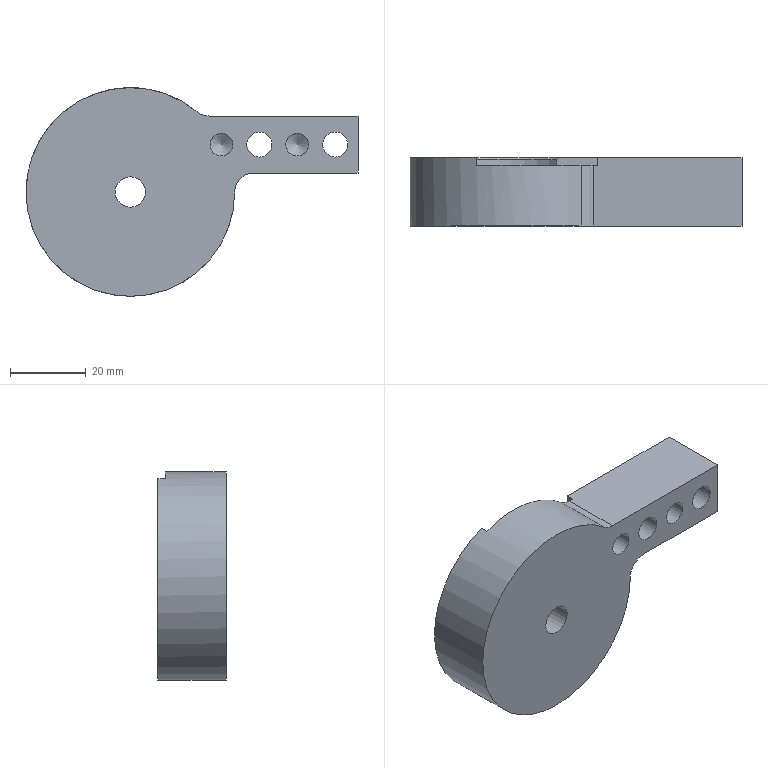Part | NX | features BREP 1 | 1 solid | 26 faces | box 87.5 x 18 x 55 mm | volume 41559 mm3 | plane 12 | cylinder 11 | cone 3 | commonest cylinder face diameters 6 x2 6.6 x2 10 x2 11 x2 8 x1 30 x1
STEP:
#1=CARTESIAN_POINT('',(17.572,7.,21.154));
#2=VERTEX_POINT('',#1);
#3=CARTESIAN_POINT('',(20.767,7.,20.));
#4=VERTEX_POINT('',#3);
#5=CARTESIAN_POINT('',(20.767,7.,25.));
#6=DIRECTION('',(0.,-1.,0.));
#7=DIRECTION('',(0.,0.,1.));
#8=AXIS2_PLACEMENT_3D('',#5,#6,#7);
#9=CIRCLE('',#8,5.);
#10=EDGE_CURVE('',#2,#4,#9,.T.);
#11=ORIENTED_EDGE('',*,*,#10,.F.);
#12=CARTESIAN_POINT('',(17.572,-9.,21.154));
#13=VERTEX_POINT('',#12);
#14=CARTESIAN_POINT('',(17.572,9.,21.154));
#15=DIRECTION('',(0.,1.,0.));
#16=VECTOR('',#15,1000.);
#17=LINE('',#14,#16);
#18=EDGE_CURVE('',#13,#2,#17,.T.);
#19=ORIENTED_EDGE('',*,*,#18,.F.);
#20=CARTESIAN_POINT('',(20.767,-9.,20.));
#21=VERTEX_POINT('',#20);
#22=CARTESIAN_POINT('',(20.767,-9.,25.));
#23=DIRECTION('',(0.,1.,0.));
#24=DIRECTION('',(0.,0.,1.));
#25=AXIS2_PLACEMENT_3D('',#22,#23,#24);
#26=CIRCLE('',#25,5.);
#27=EDGE_CURVE('',#21,#13,#26,.T.);
#28=ORIENTED_EDGE('',*,*,#27,.F.);
#29=CARTESIAN_POINT('',(20.767,-9.,20.));
#30=DIRECTION('',(0.,-1.,0.));
#31=VECTOR('',#30,1000.);
#32=LINE('',#29,#31);
#33=EDGE_CURVE('',#4,#21,#32,.T.);
#34=ORIENTED_EDGE('',*,*,#33,.F.);
#35=EDGE_LOOP('',(#11,#19,#28,#34));
#36=FACE_BOUND('',#35,.T.);
#37=CARTESIAN_POINT('',(20.767,9.,25.));
#38=DIRECTION('',(0.,-1.,0.));
#39=DIRECTION('',(0.,0.,1.));
#40=AXIS2_PLACEMENT_3D('',#37,#38,#39);
#41=CYLINDRICAL_SURFACE('',#40,5.);
#42=ADVANCED_FACE('',(#36),#41,.F.);
#43=CARTESIAN_POINT('',(-10.,7.,25.617));
#44=VERTEX_POINT('',#43);
#45=CARTESIAN_POINT('',(0.,7.,0.));
#46=DIRECTION('',(0.,1.,0.));
#47=DIRECTION('',(0.,0.,1.));
#48=AXIS2_PLACEMENT_3D('',#45,#46,#47);
#49=CIRCLE('',#48,27.5);
#50=EDGE_CURVE('',#44,#2,#49,.T.);
#51=ORIENTED_EDGE('',*,*,#50,.F.);
#52=CARTESIAN_POINT('',(-10.,9.,25.617));
#53=VERTEX_POINT('',#52);
#54=CARTESIAN_POINT('',(-10.,9.,25.617));
#55=DIRECTION('',(0.,1.,0.));
#56=VECTOR('',#55,1000.);
#57=LINE('',#54,#56);
#58=EDGE_CURVE('',#44,#53,#57,.T.);
#59=ORIENTED_EDGE('',*,*,#58,.T.);
#60=CARTESIAN_POINT('',(27.5,9.,0.));
#61=VERTEX_POINT('',#60);
#62=CARTESIAN_POINT('',(0.,9.,0.));
#63=DIRECTION('',(0.,1.,0.));
#64=DIRECTION('',(0.,0.,1.));
#65=AXIS2_PLACEMENT_3D('',#62,#63,#64);
#66=CIRCLE('',#65,27.5);
#67=EDGE_CURVE('',#61,#53,#66,.T.);
#68=ORIENTED_EDGE('',*,*,#67,.F.);
#69=CARTESIAN_POINT('',(27.5,-9.,0.));
#70=VERTEX_POINT('',#69);
#71=CARTESIAN_POINT('',(27.5,9.,0.));
#72=DIRECTION('',(0.,-1.,0.));
#73=VECTOR('',#72,1000.);
#74=LINE('',#71,#73);
#75=EDGE_CURVE('',#61,#70,#74,.T.);
#76=ORIENTED_EDGE('',*,*,#75,.T.);
#77=CARTESIAN_POINT('',(0.,-9.,0.));
#78=DIRECTION('',(0.,1.,0.));
#79=DIRECTION('',(0.,0.,1.));
#80=AXIS2_PLACEMENT_3D('',#77,#78,#79);
#81=CIRCLE('',#80,27.5);
#82=EDGE_CURVE('',#70,#13,#81,.T.);
#83=ORIENTED_EDGE('',*,*,#82,.T.);
#84=ORIENTED_EDGE('',*,*,#18,.T.);
#85=EDGE_LOOP('',(#51,#59,#68,#76,#83,#84));
#86=FACE_BOUND('',#85,.T.);
#87=CARTESIAN_POINT('',(0.,9.,0.));
#88=DIRECTION('',(0.,-1.,0.));
#89=DIRECTION('',(0.,0.,1.));
#90=AXIS2_PLACEMENT_3D('',#87,#88,#89);
#91=CYLINDRICAL_SURFACE('',#90,27.5);
#92=ADVANCED_FACE('',(#86),#91,.T.);
#93=CARTESIAN_POINT('',(-10.,9.,11.843));
#94=VERTEX_POINT('',#93);
#95=CARTESIAN_POINT('',(-10.,9.,10.));
#96=DIRECTION('',(0.,0.,1.));
#97=VECTOR('',#96,1000.);
#98=LINE('',#95,#97);
#99=EDGE_CURVE('',#94,#53,#98,.T.);
#100=ORIENTED_EDGE('',*,*,#99,.F.);
#101=CARTESIAN_POINT('',(11.843,9.,10.));
#102=VERTEX_POINT('',#101);
#103=CARTESIAN_POINT('',(0.,9.,0.));
#104=DIRECTION('',(0.,-1.,0.));
#105=DIRECTION('',(0.,0.,1.));
#106=AXIS2_PLACEMENT_3D('',#103,#104,#105);
#107=CIRCLE('',#106,15.5);
#108=EDGE_CURVE('',#94,#102,#107,.T.);
#109=ORIENTED_EDGE('',*,*,#108,.T.);
#110=CARTESIAN_POINT('',(22.,9.,10.));
#111=VERTEX_POINT('',#110);
#112=CARTESIAN_POINT('',(-10.,9.,10.));
#113=DIRECTION('',(-1.,0.,0.));
#114=VECTOR('',#113,1000.);
#115=LINE('',#112,#114);
#116=EDGE_CURVE('',#111,#102,#115,.T.);
#117=ORIENTED_EDGE('',*,*,#116,.F.);
#118=CARTESIAN_POINT('',(22.,9.,20.));
#119=VERTEX_POINT('',#118);
#120=CARTESIAN_POINT('',(22.,9.,10.));
#121=DIRECTION('',(0.,0.,-1.));
#122=VECTOR('',#121,1000.);
#123=LINE('',#120,#122);
#124=EDGE_CURVE('',#119,#111,#123,.T.);
#125=ORIENTED_EDGE('',*,*,#124,.F.);
#126=CARTESIAN_POINT('',(60.,9.,20.));
#127=VERTEX_POINT('',#126);
#128=CARTESIAN_POINT('',(0.,9.,20.));
#129=DIRECTION('',(1.,0.,0.));
#130=VECTOR('',#129,1000.);
#131=LINE('',#128,#130);
#132=EDGE_CURVE('',#119,#127,#131,.T.);
#133=ORIENTED_EDGE('',*,*,#132,.T.);
#134=CARTESIAN_POINT('',(60.,9.,5.));
#135=VERTEX_POINT('',#134);
#136=CARTESIAN_POINT('',(60.,9.,0.));
#137=DIRECTION('',(0.,0.,1.));
#138=VECTOR('',#137,1000.);
#139=LINE('',#136,#138);
#140=EDGE_CURVE('',#135,#127,#139,.T.);
#141=ORIENTED_EDGE('',*,*,#140,.F.);
#142=CARTESIAN_POINT('',(32.5,9.,5.));
#143=VERTEX_POINT('',#142);
#144=CARTESIAN_POINT('',(0.,9.,5.));
#145=DIRECTION('',(1.,0.,0.));
#146=VECTOR('',#145,1000.);
#147=LINE('',#144,#146);
#148=EDGE_CURVE('',#143,#135,#147,.T.);
#149=ORIENTED_EDGE('',*,*,#148,.F.);
#150=CARTESIAN_POINT('',(32.5,9.,0.));
#151=DIRECTION('',(0.,-1.,0.));
#152=DIRECTION('',(0.,0.,1.));
#153=AXIS2_PLACEMENT_3D('',#150,#151,#152);
#154=CIRCLE('',#153,5.);
#155=EDGE_CURVE('',#143,#61,#154,.T.);
#156=ORIENTED_EDGE('',*,*,#155,.T.);
#157=ORIENTED_EDGE('',*,*,#67,.T.);
#158=EDGE_LOOP('',(#100,#109,#117,#125,#133,#141,#149,#156,#157));
#159=FACE_BOUND('',#158,.T.);
#160=CARTESIAN_POINT('',(34.,9.,18.));
#161=VERTEX_POINT('',#160);
#162=CARTESIAN_POINT('',(34.,9.,12.5));
#163=DIRECTION('',(0.,1.,0.));
#164=DIRECTION('',(0.,0.,1.));
#165=AXIS2_PLACEMENT_3D('',#162,#163,#164);
#166=CIRCLE('',#165,5.5);
#167=EDGE_CURVE('',#161,#161,#166,.T.);
#168=ORIENTED_EDGE('',*,*,#167,.F.);
#169=EDGE_LOOP('',(#168));
#170=FACE_BOUND('',#169,.T.);
#171=CARTESIAN_POINT('',(54.,9.,18.));
#172=VERTEX_POINT('',#171);
#173=CARTESIAN_POINT('',(54.,9.,12.5));
#174=DIRECTION('',(0.,1.,0.));
#175=DIRECTION('',(0.,0.,1.));
#176=AXIS2_PLACEMENT_3D('',#173,#174,#175);
#177=CIRCLE('',#176,5.5);
#178=EDGE_CURVE('',#172,#172,#177,.T.);
#179=ORIENTED_EDGE('',*,*,#178,.F.);
#180=EDGE_LOOP('',(#179));
#181=FACE_BOUND('',#180,.T.);
#182=CARTESIAN_POINT('',(0.,9.,0.));
#183=DIRECTION('',(0.,1.,0.));
#184=DIRECTION('',(0.,0.,-1.));
#185=AXIS2_PLACEMENT_3D('',#182,#183,#184);
#186=PLANE('',#185);
#187=ADVANCED_FACE('',(#159,#170,#181),#186,.T.);
#188=CARTESIAN_POINT('',(44.,-9.,9.5));
#189=VERTEX_POINT('',#188);
#190=CARTESIAN_POINT('',(44.,-9.,12.5));
#191=DIRECTION('',(0.,-1.,0.));
#192=DIRECTION('',(0.,0.,-1.));
#193=AXIS2_PLACEMENT_3D('',#190,#191,#192);
#194=CIRCLE('',#193,3.);
#195=EDGE_CURVE('',#189,#189,#194,.T.);
#196=ORIENTED_EDGE('',*,*,#195,.F.);
#197=EDGE_LOOP('',(#196));
#198=FACE_BOUND('',#197,.T.);
#199=CARTESIAN_POINT('',(24.,-9.,9.5));
#200=VERTEX_POINT('',#199);
#201=CARTESIAN_POINT('',(24.,-9.,12.5));
#202=DIRECTION('',(0.,-1.,0.));
#203=DIRECTION('',(0.,0.,-1.));
#204=AXIS2_PLACEMENT_3D('',#201,#202,#203);
#205=CIRCLE('',#204,3.);
#206=EDGE_CURVE('',#200,#200,#205,.T.);
#207=ORIENTED_EDGE('',*,*,#206,.F.);
#208=EDGE_LOOP('',(#207));
#209=FACE_BOUND('',#208,.T.);
#210=CARTESIAN_POINT('',(34.,-9.,15.8));
#211=VERTEX_POINT('',#210);
#212=CARTESIAN_POINT('',(34.,-9.,12.5));
#213=DIRECTION('',(0.,1.,0.));
#214=DIRECTION('',(0.,0.,1.));
#215=AXIS2_PLACEMENT_3D('',#212,#213,#214);
#216=CIRCLE('',#215,3.3);
#217=EDGE_CURVE('',#211,#211,#216,.T.);
#218=ORIENTED_EDGE('',*,*,#217,.T.);
#219=EDGE_LOOP('',(#218));
#220=FACE_BOUND('',#219,.T.);
#221=CARTESIAN_POINT('',(54.,-9.,15.8));
#222=VERTEX_POINT('',#221);
#223=CARTESIAN_POINT('',(54.,-9.,12.5));
#224=DIRECTION('',(0.,1.,0.));
#225=DIRECTION('',(0.,0.,1.));
#226=AXIS2_PLACEMENT_3D('',#223,#224,#225);
#227=CIRCLE('',#226,3.3);
#228=EDGE_CURVE('',#222,#222,#227,.T.);
#229=ORIENTED_EDGE('',*,*,#228,.T.);
#230=EDGE_LOOP('',(#229));
#231=FACE_BOUND('',#230,.T.);
#232=CARTESIAN_POINT('',(0.,-9.,4.));
#233=VERTEX_POINT('',#232);
#234=CARTESIAN_POINT('',(0.,-9.,0.));
#235=DIRECTION('',(0.,1.,0.));
#236=DIRECTION('',(0.,0.,1.));
#237=AXIS2_PLACEMENT_3D('',#234,#235,#236);
#238=CIRCLE('',#237,4.);
#239=EDGE_CURVE('',#233,#233,#238,.T.);
#240=ORIENTED_EDGE('',*,*,#239,.T.);
#241=EDGE_LOOP('',(#240));
#242=FACE_BOUND('',#241,.T.);
#243=ORIENTED_EDGE('',*,*,#82,.F.);
#244=CARTESIAN_POINT('',(32.5,-9.,5.));
#245=VERTEX_POINT('',#244);
#246=CARTESIAN_POINT('',(32.5,-9.,0.));
#247=DIRECTION('',(0.,1.,0.));
#248=DIRECTION('',(0.,0.,1.));
#249=AXIS2_PLACEMENT_3D('',#246,#247,#248);
#250=CIRCLE('',#249,5.);
#251=EDGE_CURVE('',#70,#245,#250,.T.);
#252=ORIENTED_EDGE('',*,*,#251,.T.);
#253=CARTESIAN_POINT('',(60.,-9.,5.));
#254=VERTEX_POINT('',#253);
#255=CARTESIAN_POINT('',(0.,-9.,5.));
#256=DIRECTION('',(1.,0.,0.));
#257=VECTOR('',#256,1000.);
#258=LINE('',#255,#257);
#259=EDGE_CURVE('',#245,#254,#258,.T.);
#260=ORIENTED_EDGE('',*,*,#259,.T.);
#261=CARTESIAN_POINT('',(60.,-9.,20.));
#262=VERTEX_POINT('',#261);
#263=CARTESIAN_POINT('',(60.,-9.,0.));
#264=DIRECTION('',(0.,0.,1.));
#265=VECTOR('',#264,1000.);
#266=LINE('',#263,#265);
#267=EDGE_CURVE('',#254,#262,#266,.T.);
#268=ORIENTED_EDGE('',*,*,#267,.T.);
#269=CARTESIAN_POINT('',(0.,-9.,20.));
#270=DIRECTION('',(1.,0.,0.));
#271=VECTOR('',#270,1000.);
#272=LINE('',#269,#271);
#273=EDGE_CURVE('',#21,#262,#272,.T.);
#274=ORIENTED_EDGE('',*,*,#273,.F.);
#275=ORIENTED_EDGE('',*,*,#27,.T.);
#276=EDGE_LOOP('',(#243,#252,#260,#268,#274,#275));
#277=FACE_BOUND('',#276,.T.);
#278=CARTESIAN_POINT('',(0.,-9.,0.));
#279=DIRECTION('',(0.,1.,0.));
#280=DIRECTION('',(0.,0.,-1.));
#281=AXIS2_PLACEMENT_3D('',#278,#279,#280);
#282=PLANE('',#281);
#283=ADVANCED_FACE('',(#198,#209,#220,#231,#242,#277),#282,.F.);
#284=CARTESIAN_POINT('',(60.,52.776,5.));
#285=DIRECTION('',(0.,-1.,0.));
#286=VECTOR('',#285,1000.);
#287=LINE('',#284,#286);
#288=EDGE_CURVE('',#135,#254,#287,.T.);
#289=ORIENTED_EDGE('',*,*,#288,.F.);
#290=ORIENTED_EDGE('',*,*,#140,.T.);
#291=CARTESIAN_POINT('',(60.,52.776,20.));
#292=DIRECTION('',(0.,-1.,0.));
#293=VECTOR('',#292,1000.);
#294=LINE('',#291,#293);
#295=EDGE_CURVE('',#127,#262,#294,.T.);
#296=ORIENTED_EDGE('',*,*,#295,.T.);
#297=ORIENTED_EDGE('',*,*,#267,.F.);
#298=EDGE_LOOP('',(#289,#290,#296,#297));
#299=FACE_BOUND('',#298,.T.);
#300=CARTESIAN_POINT('',(60.,52.776,0.));
#301=DIRECTION('',(1.,0.,0.));
#302=DIRECTION('',(0.,0.,1.));
#303=AXIS2_PLACEMENT_3D('',#300,#301,#302);
#304=PLANE('',#303);
#305=ADVANCED_FACE('',(#299),#304,.T.);
#306=ORIENTED_EDGE('',*,*,#132,.F.);
#307=CARTESIAN_POINT('',(22.,7.,20.));
#308=VERTEX_POINT('',#307);
#309=CARTESIAN_POINT('',(22.,52.776,20.));
#310=DIRECTION('',(0.,-1.,0.));
#311=VECTOR('',#310,1000.);
#312=LINE('',#309,#311);
#313=EDGE_CURVE('',#119,#308,#312,.T.);
#314=ORIENTED_EDGE('',*,*,#313,.T.);
#315=CARTESIAN_POINT('',(0.,7.,20.));
#316=DIRECTION('',(1.,0.,0.));
#317=VECTOR('',#316,1000.);
#318=LINE('',#315,#317);
#319=EDGE_CURVE('',#4,#308,#318,.T.);
#320=ORIENTED_EDGE('',*,*,#319,.F.);
#321=ORIENTED_EDGE('',*,*,#33,.T.);
#322=ORIENTED_EDGE('',*,*,#273,.T.);
#323=ORIENTED_EDGE('',*,*,#295,.F.);
#324=EDGE_LOOP('',(#306,#314,#320,#321,#322,#323));
#325=FACE_BOUND('',#324,.T.);
#326=CARTESIAN_POINT('',(0.,52.776,20.));
#327=DIRECTION('',(0.,0.,-1.));
#328=DIRECTION('',(1.,0.,0.));
#329=AXIS2_PLACEMENT_3D('',#326,#327,#328);
#330=PLANE('',#329);
#331=ADVANCED_FACE('',(#325),#330,.F.);
#332=ORIENTED_EDGE('',*,*,#259,.F.);
#333=CARTESIAN_POINT('',(32.5,52.776,5.));
#334=DIRECTION('',(0.,1.,0.));
#335=VECTOR('',#334,1000.);
#336=LINE('',#333,#335);
#337=EDGE_CURVE('',#245,#143,#336,.T.);
#338=ORIENTED_EDGE('',*,*,#337,.T.);
#339=ORIENTED_EDGE('',*,*,#148,.T.);
#340=ORIENTED_EDGE('',*,*,#288,.T.);
#341=EDGE_LOOP('',(#332,#338,#339,#340));
#342=FACE_BOUND('',#341,.T.);
#343=CARTESIAN_POINT('',(0.,52.776,5.));
#344=DIRECTION('',(0.,0.,-1.));
#345=DIRECTION('',(1.,0.,0.));
#346=AXIS2_PLACEMENT_3D('',#343,#344,#345);
#347=PLANE('',#346);
#348=ADVANCED_FACE('',(#342),#347,.T.);
#349=CARTESIAN_POINT('',(11.18,8.5,10.));
#350=VERTEX_POINT('',#349);
#351=CARTESIAN_POINT('',(-10.,8.5,11.18));
#352=VERTEX_POINT('',#351);
#353=CARTESIAN_POINT('',(0.,8.5,0.));
#354=DIRECTION('',(0.,1.,0.));
#355=DIRECTION('',(0.,0.,1.));
#356=AXIS2_PLACEMENT_3D('',#353,#354,#355);
#357=CIRCLE('',#356,15.);
#358=EDGE_CURVE('',#350,#352,#357,.T.);
#359=ORIENTED_EDGE('',*,*,#358,.T.);
#360=CARTESIAN_POINT('',(-10.,7.,11.18));
#361=VERTEX_POINT('',#360);
#362=CARTESIAN_POINT('',(-10.,-1.,11.18));
#363=DIRECTION('',(0.,-1.,0.));
#364=VECTOR('',#363,1000.);
#365=LINE('',#362,#364);
#366=EDGE_CURVE('',#352,#361,#365,.T.);
#367=ORIENTED_EDGE('',*,*,#366,.T.);
#368=CARTESIAN_POINT('',(11.18,7.,10.));
#369=VERTEX_POINT('',#368);
#370=CARTESIAN_POINT('',(0.,7.,0.));
#371=DIRECTION('',(0.,-1.,0.));
#372=DIRECTION('',(0.,0.,1.));
#373=AXIS2_PLACEMENT_3D('',#370,#371,#372);
#374=CIRCLE('',#373,15.);
#375=EDGE_CURVE('',#369,#361,#374,.T.);
#376=ORIENTED_EDGE('',*,*,#375,.F.);
#377=CARTESIAN_POINT('',(11.18,-1.,10.));
#378=DIRECTION('',(0.,1.,0.));
#379=VECTOR('',#378,1000.);
#380=LINE('',#377,#379);
#381=EDGE_CURVE('',#369,#350,#380,.T.);
#382=ORIENTED_EDGE('',*,*,#381,.T.);
#383=EDGE_LOOP('',(#359,#367,#376,#382));
#384=FACE_BOUND('',#383,.T.);
#385=CARTESIAN_POINT('',(0.,-1.,15.));
#386=VERTEX_POINT('',#385);
#387=CARTESIAN_POINT('',(0.,-1.,0.));
#388=DIRECTION('',(0.,1.,0.));
#389=DIRECTION('',(0.,0.,1.));
#390=AXIS2_PLACEMENT_3D('',#387,#388,#389);
#391=CIRCLE('',#390,15.);
#392=EDGE_CURVE('',#386,#386,#391,.T.);
#393=ORIENTED_EDGE('',*,*,#392,.F.);
#394=EDGE_LOOP('',(#393));
#395=FACE_BOUND('',#394,.T.);
#396=CARTESIAN_POINT('',(0.,-1.,0.));
#397=DIRECTION('',(0.,1.,0.));
#398=DIRECTION('',(0.,0.,-1.));
#399=AXIS2_PLACEMENT_3D('',#396,#397,#398);
#400=CYLINDRICAL_SURFACE('',#399,15.);
#401=ADVANCED_FACE('',(#384,#395),#400,.F.);
#402=CARTESIAN_POINT('',(0.,-1.,4.));
#403=VERTEX_POINT('',#402);
#404=CARTESIAN_POINT('',(0.,-1.,0.));
#405=DIRECTION('',(0.,1.,0.));
#406=DIRECTION('',(0.,0.,1.));
#407=AXIS2_PLACEMENT_3D('',#404,#405,#406);
#408=CIRCLE('',#407,4.);
#409=EDGE_CURVE('',#403,#403,#408,.T.);
#410=ORIENTED_EDGE('',*,*,#409,.F.);
#411=EDGE_LOOP('',(#410));
#412=FACE_BOUND('',#411,.T.);
#413=ORIENTED_EDGE('',*,*,#392,.T.);
#414=EDGE_LOOP('',(#413));
#415=FACE_BOUND('',#414,.T.);
#416=CARTESIAN_POINT('',(0.,-1.,0.));
#417=DIRECTION('',(0.,1.,0.));
#418=DIRECTION('',(0.,0.,-1.));
#419=AXIS2_PLACEMENT_3D('',#416,#417,#418);
#420=PLANE('',#419);
#421=ADVANCED_FACE('',(#412,#415),#420,.T.);
#422=ORIENTED_EDGE('',*,*,#239,.F.);
#423=EDGE_LOOP('',(#422));
#424=FACE_BOUND('',#423,.T.);
#425=ORIENTED_EDGE('',*,*,#409,.T.);
#426=EDGE_LOOP('',(#425));
#427=FACE_BOUND('',#426,.T.);
#428=CARTESIAN_POINT('',(0.,-1.,0.));
#429=DIRECTION('',(0.,1.,0.));
#430=DIRECTION('',(0.,0.,-1.));
#431=AXIS2_PLACEMENT_3D('',#428,#429,#430);
#432=CYLINDRICAL_SURFACE('',#431,4.);
#433=ADVANCED_FACE('',(#424,#427),#432,.F.);
#434=ORIENTED_EDGE('',*,*,#228,.F.);
#435=EDGE_LOOP('',(#434));
#436=FACE_BOUND('',#435,.T.);
#437=CARTESIAN_POINT('',(54.,2.6,15.8));
#438=VERTEX_POINT('',#437);
#439=CARTESIAN_POINT('',(54.,2.6,12.5));
#440=DIRECTION('',(0.,1.,0.));
#441=DIRECTION('',(0.,0.,1.));
#442=AXIS2_PLACEMENT_3D('',#439,#440,#441);
#443=CIRCLE('',#442,3.3);
#444=EDGE_CURVE('',#438,#438,#443,.T.);
#445=ORIENTED_EDGE('',*,*,#444,.T.);
#446=EDGE_LOOP('',(#445));
#447=FACE_BOUND('',#446,.T.);
#448=CARTESIAN_POINT('',(54.,9.,12.5));
#449=DIRECTION('',(0.,1.,0.));
#450=DIRECTION('',(0.,0.,-1.));
#451=AXIS2_PLACEMENT_3D('',#448,#449,#450);
#452=CYLINDRICAL_SURFACE('',#451,3.3);
#453=ADVANCED_FACE('',(#436,#447),#452,.F.);
#454=ORIENTED_EDGE('',*,*,#444,.F.);
#455=EDGE_LOOP('',(#454));
#456=FACE_BOUND('',#455,.T.);
#457=CARTESIAN_POINT('',(54.,2.6,18.));
#458=VERTEX_POINT('',#457);
#459=CARTESIAN_POINT('',(54.,2.6,12.5));
#460=DIRECTION('',(0.,1.,0.));
#461=DIRECTION('',(0.,0.,1.));
#462=AXIS2_PLACEMENT_3D('',#459,#460,#461);
#463=CIRCLE('',#462,5.5);
#464=EDGE_CURVE('',#458,#458,#463,.T.);
#465=ORIENTED_EDGE('',*,*,#464,.T.);
#466=EDGE_LOOP('',(#465));
#467=FACE_BOUND('',#466,.T.);
#468=CARTESIAN_POINT('',(57.3,2.6,12.5));
#469=DIRECTION('',(0.,-1.,0.));
#470=DIRECTION('',(0.,0.,1.));
#471=AXIS2_PLACEMENT_3D('',#468,#469,#470);
#472=PLANE('',#471);
#473=ADVANCED_FACE('',(#456,#467),#472,.F.);
#474=ORIENTED_EDGE('',*,*,#464,.F.);
#475=EDGE_LOOP('',(#474));
#476=FACE_BOUND('',#475,.T.);
#477=ORIENTED_EDGE('',*,*,#178,.T.);
#478=EDGE_LOOP('',(#477));
#479=FACE_BOUND('',#478,.T.);
#480=CARTESIAN_POINT('',(54.,9.,12.5));
#481=DIRECTION('',(0.,1.,0.));
#482=DIRECTION('',(0.,0.,-1.));
#483=AXIS2_PLACEMENT_3D('',#480,#481,#482);
#484=CYLINDRICAL_SURFACE('',#483,5.5);
#485=ADVANCED_FACE('',(#476,#479),#484,.F.);
#486=ORIENTED_EDGE('',*,*,#217,.F.);
#487=EDGE_LOOP('',(#486));
#488=FACE_BOUND('',#487,.T.);
#489=CARTESIAN_POINT('',(34.,2.6,15.8));
#490=VERTEX_POINT('',#489);
#491=CARTESIAN_POINT('',(34.,2.6,12.5));
#492=DIRECTION('',(0.,1.,0.));
#493=DIRECTION('',(0.,0.,1.));
#494=AXIS2_PLACEMENT_3D('',#491,#492,#493);
#495=CIRCLE('',#494,3.3);
#496=EDGE_CURVE('',#490,#490,#495,.T.);
#497=ORIENTED_EDGE('',*,*,#496,.T.);
#498=EDGE_LOOP('',(#497));
#499=FACE_BOUND('',#498,.T.);
#500=CARTESIAN_POINT('',(34.,9.,12.5));
#501=DIRECTION('',(0.,1.,0.));
#502=DIRECTION('',(0.,0.,-1.));
#503=AXIS2_PLACEMENT_3D('',#500,#501,#502);
#504=CYLINDRICAL_SURFACE('',#503,3.3);
#505=ADVANCED_FACE('',(#488,#499),#504,.F.);
#506=ORIENTED_EDGE('',*,*,#496,.F.);
#507=EDGE_LOOP('',(#506));
#508=FACE_BOUND('',#507,.T.);
#509=CARTESIAN_POINT('',(34.,2.6,18.));
#510=VERTEX_POINT('',#509);
#511=CARTESIAN_POINT('',(34.,2.6,12.5));
#512=DIRECTION('',(0.,1.,0.));
#513=DIRECTION('',(0.,0.,1.));
#514=AXIS2_PLACEMENT_3D('',#511,#512,#513);
#515=CIRCLE('',#514,5.5);
#516=EDGE_CURVE('',#510,#510,#515,.T.);
#517=ORIENTED_EDGE('',*,*,#516,.T.);
#518=EDGE_LOOP('',(#517));
#519=FACE_BOUND('',#518,.T.);
#520=CARTESIAN_POINT('',(37.3,2.6,12.5));
#521=DIRECTION('',(0.,-1.,0.));
#522=DIRECTION('',(0.,0.,1.));
#523=AXIS2_PLACEMENT_3D('',#520,#521,#522);
#524=PLANE('',#523);
#525=ADVANCED_FACE('',(#508,#519),#524,.F.);
#526=ORIENTED_EDGE('',*,*,#516,.F.);
#527=EDGE_LOOP('',(#526));
#528=FACE_BOUND('',#527,.T.);
#529=ORIENTED_EDGE('',*,*,#167,.T.);
#530=EDGE_LOOP('',(#529));
#531=FACE_BOUND('',#530,.T.);
#532=CARTESIAN_POINT('',(34.,9.,12.5));
#533=DIRECTION('',(0.,1.,0.));
#534=DIRECTION('',(0.,0.,-1.));
#535=AXIS2_PLACEMENT_3D('',#532,#533,#534);
#536=CYLINDRICAL_SURFACE('',#535,5.5);
#537=ADVANCED_FACE('',(#528,#531),#536,.F.);
#538=CARTESIAN_POINT('',(24.,5.203,12.5));
#539=VERTEX_POINT('',#538);
#540=VERTEX_LOOP('',#539);
#541=FACE_BOUND('',#540,.T.);
#542=CARTESIAN_POINT('',(24.,3.4,9.5));
#543=VERTEX_POINT('',#542);
#544=CARTESIAN_POINT('',(24.,3.4,12.5));
#545=DIRECTION('',(0.,-1.,0.));
#546=DIRECTION('',(0.,0.,-1.));
#547=AXIS2_PLACEMENT_3D('',#544,#545,#546);
#548=CIRCLE('',#547,3.);
#549=EDGE_CURVE('',#543,#543,#548,.T.);
#550=ORIENTED_EDGE('',*,*,#549,.T.);
#551=EDGE_LOOP('',(#550));
#552=FACE_BOUND('',#551,.T.);
#553=CARTESIAN_POINT('',(24.,3.4,12.5));
#554=DIRECTION('',(0.,-1.,0.));
#555=DIRECTION('',(0.,0.,1.));
#556=AXIS2_PLACEMENT_3D('',#553,#554,#555);
#557=CONICAL_SURFACE('',#556,3.,1.03);
#558=ADVANCED_FACE('',(#541,#552),#557,.F.);
#559=ORIENTED_EDGE('',*,*,#549,.F.);
#560=EDGE_LOOP('',(#559));
#561=FACE_BOUND('',#560,.T.);
#562=ORIENTED_EDGE('',*,*,#206,.T.);
#563=EDGE_LOOP('',(#562));
#564=FACE_BOUND('',#563,.T.);
#565=CARTESIAN_POINT('',(24.,-9.,12.5));
#566=DIRECTION('',(0.,-1.,0.));
#567=DIRECTION('',(0.,0.,1.));
#568=AXIS2_PLACEMENT_3D('',#565,#566,#567);
#569=CYLINDRICAL_SURFACE('',#568,3.);
#570=ADVANCED_FACE('',(#561,#564),#569,.F.);
#571=CARTESIAN_POINT('',(44.,5.203,12.5));
#572=VERTEX_POINT('',#571);
#573=VERTEX_LOOP('',#572);
#574=FACE_BOUND('',#573,.T.);
#575=CARTESIAN_POINT('',(44.,3.4,9.5));
#576=VERTEX_POINT('',#575);
#577=CARTESIAN_POINT('',(44.,3.4,12.5));
#578=DIRECTION('',(0.,-1.,0.));
#579=DIRECTION('',(0.,0.,-1.));
#580=AXIS2_PLACEMENT_3D('',#577,#578,#579);
#581=CIRCLE('',#580,3.);
#582=EDGE_CURVE('',#576,#576,#581,.T.);
#583=ORIENTED_EDGE('',*,*,#582,.T.);
#584=EDGE_LOOP('',(#583));
#585=FACE_BOUND('',#584,.T.);
#586=CARTESIAN_POINT('',(44.,3.4,12.5));
#587=DIRECTION('',(0.,-1.,0.));
#588=DIRECTION('',(0.,0.,1.));
#589=AXIS2_PLACEMENT_3D('',#586,#587,#588);
#590=CONICAL_SURFACE('',#589,3.,1.03);
#591=ADVANCED_FACE('',(#574,#585),#590,.F.);
#592=ORIENTED_EDGE('',*,*,#582,.F.);
#593=EDGE_LOOP('',(#592));
#594=FACE_BOUND('',#593,.T.);
#595=ORIENTED_EDGE('',*,*,#195,.T.);
#596=EDGE_LOOP('',(#595));
#597=FACE_BOUND('',#596,.T.);
#598=CARTESIAN_POINT('',(44.,-9.,12.5));
#599=DIRECTION('',(0.,-1.,0.));
#600=DIRECTION('',(0.,0.,1.));
#601=AXIS2_PLACEMENT_3D('',#598,#599,#600);
#602=CYLINDRICAL_SURFACE('',#601,3.);
#603=ADVANCED_FACE('',(#594,#597),#602,.F.);
#604=ORIENTED_EDGE('',*,*,#155,.F.);
#605=ORIENTED_EDGE('',*,*,#337,.F.);
#606=ORIENTED_EDGE('',*,*,#251,.F.);
#607=ORIENTED_EDGE('',*,*,#75,.F.);
#608=EDGE_LOOP('',(#604,#605,#606,#607));
#609=FACE_BOUND('',#608,.T.);
#610=CARTESIAN_POINT('',(32.5,9.,0.));
#611=DIRECTION('',(0.,-1.,0.));
#612=DIRECTION('',(0.,0.,1.));
#613=AXIS2_PLACEMENT_3D('',#610,#611,#612);
#614=CYLINDRICAL_SURFACE('',#613,5.);
#615=ADVANCED_FACE('',(#609),#614,.F.);
#616=CARTESIAN_POINT('',(-10.,8.5,11.18));
#617=CARTESIAN_POINT('',(-10.,8.665,11.402));
#618=CARTESIAN_POINT('',(-10.,8.832,11.623));
#619=CARTESIAN_POINT('',(-10.,9.,11.843));
#620=B_SPLINE_CURVE_WITH_KNOTS('',3,(#616,#617,#618,#619),.UNSPECIFIED.,.F.,.F.,(4,4),(0.,1.),.PIECEWISE_BEZIER_KNOTS.);
#621=EDGE_CURVE('',#352,#94,#620,.T.);
#622=ORIENTED_EDGE('',*,*,#621,.F.);
#623=ORIENTED_EDGE('',*,*,#358,.F.);
#624=CARTESIAN_POINT('',(11.843,9.,10.));
#625=CARTESIAN_POINT('',(11.623,8.832,10.));
#626=CARTESIAN_POINT('',(11.402,8.665,10.));
#627=CARTESIAN_POINT('',(11.18,8.5,10.));
#628=B_SPLINE_CURVE_WITH_KNOTS('',3,(#624,#625,#626,#627),.UNSPECIFIED.,.F.,.F.,(4,4),(0.,1.),.PIECEWISE_BEZIER_KNOTS.);
#629=EDGE_CURVE('',#102,#350,#628,.T.);
#630=ORIENTED_EDGE('',*,*,#629,.F.);
#631=ORIENTED_EDGE('',*,*,#108,.F.);
#632=EDGE_LOOP('',(#622,#623,#630,#631));
#633=FACE_BOUND('',#632,.T.);
#634=CARTESIAN_POINT('',(0.,8.5,0.));
#635=DIRECTION('',(0.,1.,0.));
#636=DIRECTION('',(0.,0.,-1.));
#637=AXIS2_PLACEMENT_3D('',#634,#635,#636);
#638=CONICAL_SURFACE('',#637,15.,0.7854);
#639=ADVANCED_FACE('',(#633),#638,.F.);
#640=ORIENTED_EDGE('',*,*,#124,.T.);
#641=CARTESIAN_POINT('',(22.,7.,10.));
#642=VERTEX_POINT('',#641);
#643=CARTESIAN_POINT('',(22.,7.,10.));
#644=DIRECTION('',(0.,1.,0.));
#645=VECTOR('',#644,1000.);
#646=LINE('',#643,#645);
#647=EDGE_CURVE('',#642,#111,#646,.T.);
#648=ORIENTED_EDGE('',*,*,#647,.F.);
#649=CARTESIAN_POINT('',(22.,7.,10.));
#650=DIRECTION('',(0.,0.,-1.));
#651=VECTOR('',#650,1000.);
#652=LINE('',#649,#651);
#653=EDGE_CURVE('',#308,#642,#652,.T.);
#654=ORIENTED_EDGE('',*,*,#653,.F.);
#655=ORIENTED_EDGE('',*,*,#313,.F.);
#656=EDGE_LOOP('',(#640,#648,#654,#655));
#657=FACE_BOUND('',#656,.T.);
#658=CARTESIAN_POINT('',(22.,7.,10.));
#659=DIRECTION('',(1.,0.,0.));
#660=DIRECTION('',(0.,0.,1.));
#661=AXIS2_PLACEMENT_3D('',#658,#659,#660);
#662=PLANE('',#661);
#663=ADVANCED_FACE('',(#657),#662,.F.);
#664=ORIENTED_EDGE('',*,*,#375,.T.);
#665=CARTESIAN_POINT('',(-10.,7.,10.));
#666=DIRECTION('',(0.,0.,1.));
#667=VECTOR('',#666,1000.);
#668=LINE('',#665,#667);
#669=EDGE_CURVE('',#361,#44,#668,.T.);
#670=ORIENTED_EDGE('',*,*,#669,.T.);
#671=ORIENTED_EDGE('',*,*,#50,.T.);
#672=ORIENTED_EDGE('',*,*,#10,.T.);
#673=ORIENTED_EDGE('',*,*,#319,.T.);
#674=ORIENTED_EDGE('',*,*,#653,.T.);
#675=CARTESIAN_POINT('',(-10.,7.,10.));
#676=DIRECTION('',(-1.,0.,0.));
#677=VECTOR('',#676,1000.);
#678=LINE('',#675,#677);
#679=EDGE_CURVE('',#642,#369,#678,.T.);
#680=ORIENTED_EDGE('',*,*,#679,.T.);
#681=EDGE_LOOP('',(#664,#670,#671,#672,#673,#674,#680));
#682=FACE_BOUND('',#681,.T.);
#683=CARTESIAN_POINT('',(0.,7.,0.));
#684=DIRECTION('',(0.,1.,0.));
#685=DIRECTION('',(0.,0.,-1.));
#686=AXIS2_PLACEMENT_3D('',#683,#684,#685);
#687=PLANE('',#686);
#688=ADVANCED_FACE('',(#682),#687,.T.);
#689=ORIENTED_EDGE('',*,*,#669,.F.);
#690=ORIENTED_EDGE('',*,*,#366,.F.);
#691=ORIENTED_EDGE('',*,*,#621,.T.);
#692=ORIENTED_EDGE('',*,*,#99,.T.);
#693=ORIENTED_EDGE('',*,*,#58,.F.);
#694=EDGE_LOOP('',(#689,#690,#691,#692,#693));
#695=FACE_BOUND('',#694,.T.);
#696=CARTESIAN_POINT('',(-10.,7.,10.));
#697=DIRECTION('',(-1.,0.,0.));
#698=DIRECTION('',(0.,0.,-1.));
#699=AXIS2_PLACEMENT_3D('',#696,#697,#698);
#700=PLANE('',#699);
#701=ADVANCED_FACE('',(#695),#700,.F.);
#702=ORIENTED_EDGE('',*,*,#679,.F.);
#703=ORIENTED_EDGE('',*,*,#647,.T.);
#704=ORIENTED_EDGE('',*,*,#116,.T.);
#705=ORIENTED_EDGE('',*,*,#629,.T.);
#706=ORIENTED_EDGE('',*,*,#381,.F.);
#707=EDGE_LOOP('',(#702,#703,#704,#705,#706));
#708=FACE_BOUND('',#707,.T.);
#709=CARTESIAN_POINT('',(-10.,7.,10.));
#710=DIRECTION('',(0.,0.,-1.));
#711=DIRECTION('',(1.,0.,0.));
#712=AXIS2_PLACEMENT_3D('',#709,#710,#711);
#713=PLANE('',#712);
#714=ADVANCED_FACE('',(#708),#713,.F.);
#715=CLOSED_SHELL('',(#42,#92,#187,#283,#305,#331,#348,#401,#421,#433,#453,#473,#485,#505,#525,#537,#558,#570,#591,#603,#615,#639,#663,#688,#701,#714));
#716=MANIFOLD_SOLID_BREP('',#715);
#717=(LENGTH_UNIT()NAMED_UNIT(*)SI_UNIT(.MILLI.,.METRE.));
#718=UNCERTAINTY_MEASURE_WITH_UNIT(LENGTH_MEASURE(0.00001),#717,'','');
#719=(NAMED_UNIT(*)PLANE_ANGLE_UNIT()SI_UNIT($,.RADIAN.));
#720=(NAMED_UNIT(*)SI_UNIT($,.STERADIAN.)SOLID_ANGLE_UNIT());
#721=(GEOMETRIC_REPRESENTATION_CONTEXT(3)GLOBAL_UNCERTAINTY_ASSIGNED_CONTEXT((#718))GLOBAL_UNIT_ASSIGNED_CONTEXT((#717,#719,#720))REPRESENTATION_CONTEXT('',''));
#722=ADVANCED_BREP_SHAPE_REPRESENTATION('',(#716),#721);